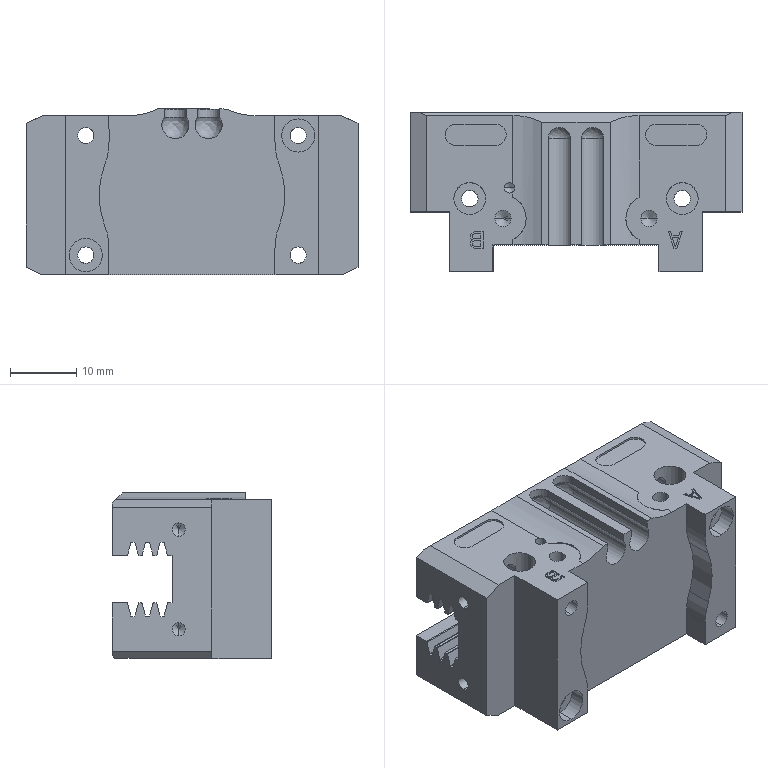Part | SolidWorks | features BaseBody 1 | 1 solid | 302 faces | box 50 x 24 x 25 mm | volume 17442 mm3 | plane 143 | cylinder 127 | cone 30 | spline 2 | commonest cylinder face diameters 2.459 x26 0.2 x24 1.567 x12 2.5 x12 4.8 x12 5 x12